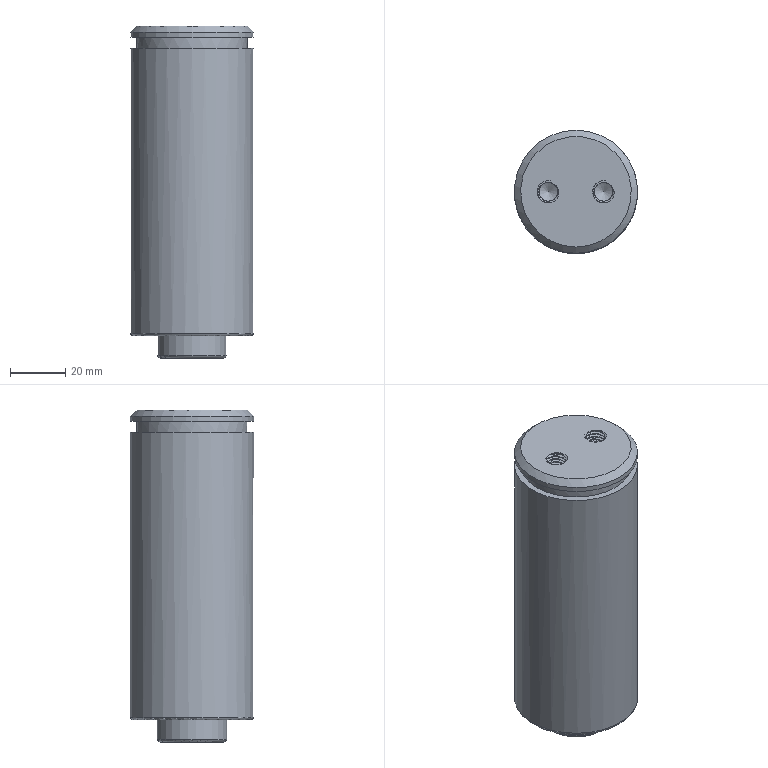Part | STEP file | 1_id1106_x_t | 1 solid | 143 faces | box 44.5 x 44.5 x 120 mm | volume 176158 mm3 | other 86 | plane 38 | cylinder 8 | spline 6 | cone 3 | torus 2 | commonest cylinder face diameters 6.8 x2 8 x2 44.5 x2 25 x1 40 x1